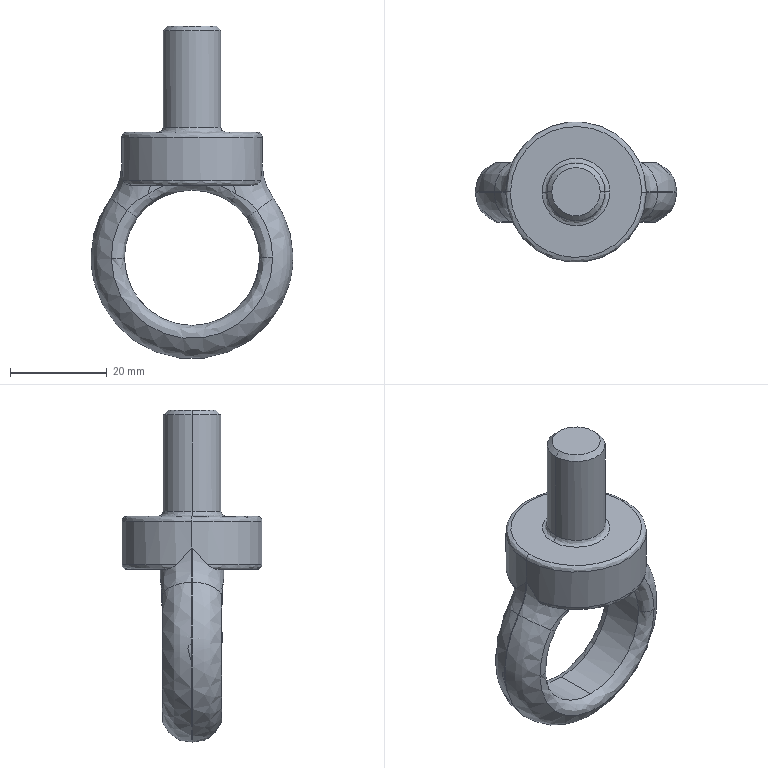Part | SolidWorks | features BaseBody 1 | 1 solid | 45 faces | box 41.795 x 29.1 x 68.897 mm | volume 16269 mm3 | spline 29 | plane 8 | cylinder 6 | cone 2 | commonest cylinder face diameters 12 x2 28 x2 29.1 x2